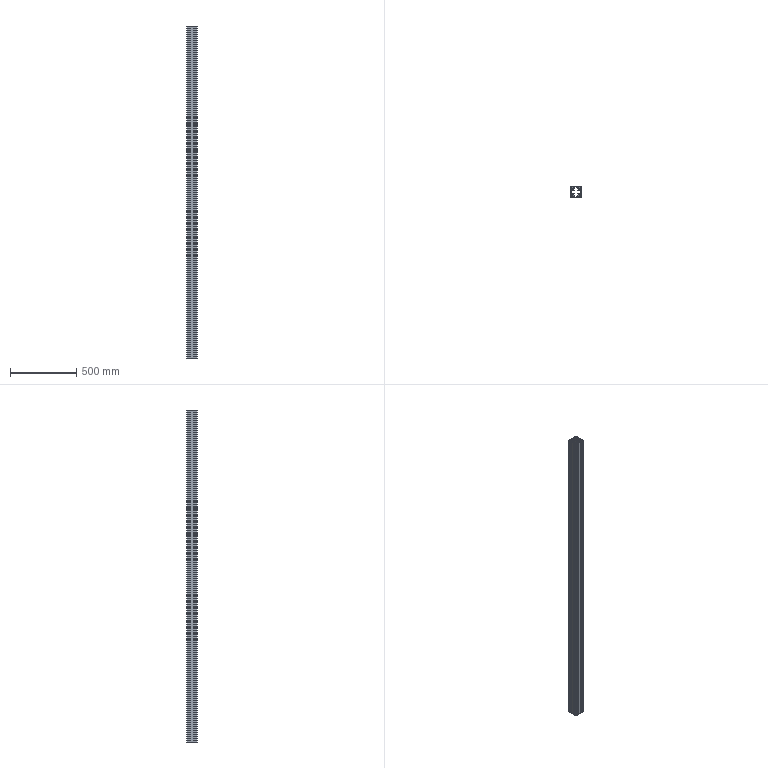Part | SolidWorks | features HoleWzd 3, ICE 3, MirrorPattern 3, Fillet 2, Extrusion 1 | 1 solid | 239 faces | box 80 x 80 x 2500 mm | volume 4298649 mm3 | plane 194 | cylinder 29 | cone 16 | commonest cylinder face diameters 6.8 x16 6.5 x8 9 x4 5 x1